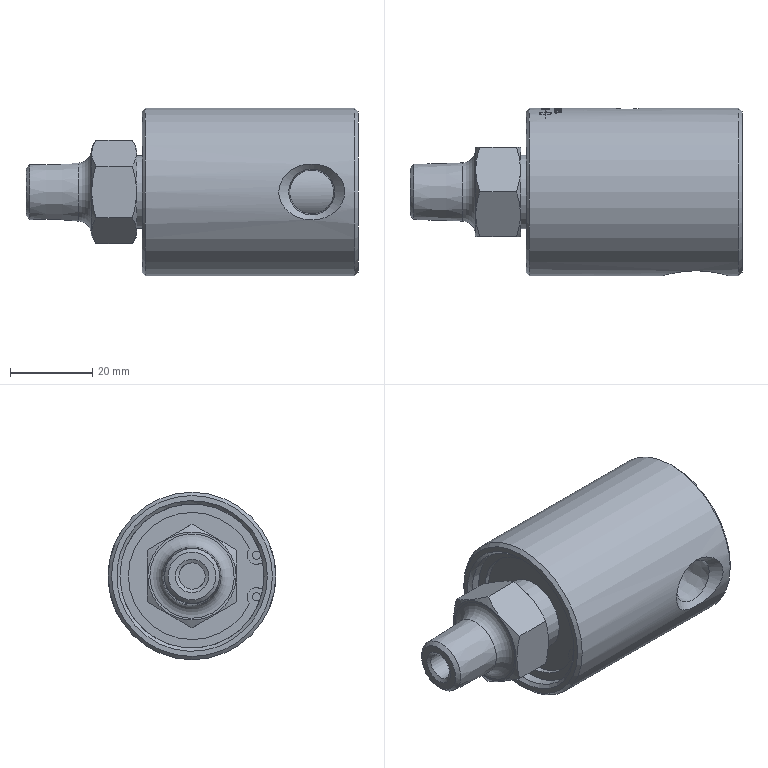Part | STEP file | 1102-070-082 | 1 solid | 337 faces | box 80.735 x 40.71 x 40.71 mm | volume 70231 mm3 | spline 175 | plane 99 | cylinder 50 | cone 11 | torus 1 | sphere 1 | commonest cylinder face diameters 40.66 x22 40.71 x13 1.981 x2 4.572 x2 15 x2 4.7 x1